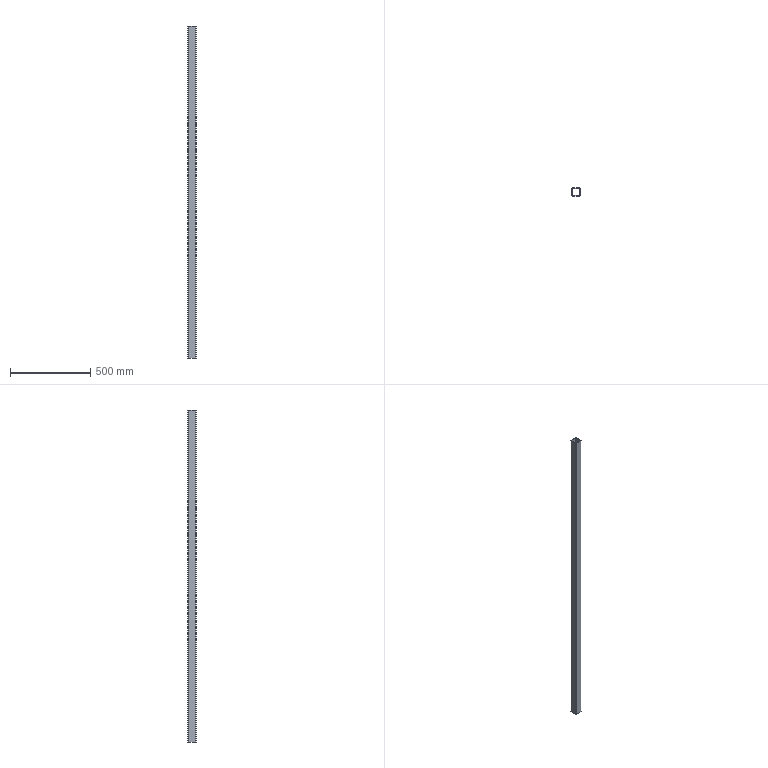Part | SolidWorks | 1 solid | 18 faces | box 50 x 50 x 2070 mm | volume 1119504 mm3 | plane 10 | cylinder 8 | commonest cylinder face diameters 6 x4 12 x4
STEP:
#1=CARTESIAN_POINT('',(19.,25.,1035.));
#2=VERTEX_POINT('',#1);
#3=CARTESIAN_POINT('',(25.,19.,1035.));
#4=VERTEX_POINT('',#3);
#5=CARTESIAN_POINT('',(19.,19.,1035.));
#6=DIRECTION('',(0.,0.,-1.));
#7=DIRECTION('',(-1.,0.,0.));
#8=AXIS2_PLACEMENT_3D('',#5,#6,#7);
#9=CIRCLE('',#8,6.);
#10=EDGE_CURVE('',#2,#4,#9,.T.);
#11=ORIENTED_EDGE('',*,*,#10,.T.);
#12=CARTESIAN_POINT('',(25.,19.,-1035.));
#13=VERTEX_POINT('',#12);
#14=CARTESIAN_POINT('',(25.,19.,-1035.));
#15=DIRECTION('',(0.,0.,1.));
#16=VECTOR('',#15,1000.);
#17=LINE('',#14,#16);
#18=EDGE_CURVE('',#13,#4,#17,.T.);
#19=ORIENTED_EDGE('',*,*,#18,.F.);
#20=CARTESIAN_POINT('',(19.,25.,-1035.));
#21=VERTEX_POINT('',#20);
#22=CARTESIAN_POINT('',(19.,19.,-1035.));
#23=DIRECTION('',(0.,0.,-1.));
#24=DIRECTION('',(-1.,0.,0.));
#25=AXIS2_PLACEMENT_3D('',#22,#23,#24);
#26=CIRCLE('',#25,6.);
#27=EDGE_CURVE('',#21,#13,#26,.T.);
#28=ORIENTED_EDGE('',*,*,#27,.F.);
#29=CARTESIAN_POINT('',(19.,25.,-1035.));
#30=DIRECTION('',(0.,0.,1.));
#31=VECTOR('',#30,1000.);
#32=LINE('',#29,#31);
#33=EDGE_CURVE('',#21,#2,#32,.T.);
#34=ORIENTED_EDGE('',*,*,#33,.T.);
#35=EDGE_LOOP('',(#11,#19,#28,#34));
#36=FACE_OUTER_BOUND('',#35,.T.);
#37=CARTESIAN_POINT('',(19.,19.,-1035.));
#38=DIRECTION('',(0.,0.,1.));
#39=DIRECTION('',(1.,0.,0.));
#40=AXIS2_PLACEMENT_3D('',#37,#38,#39);
#41=CYLINDRICAL_SURFACE('',#40,6.);
#42=ADVANCED_FACE('',(#36),#41,.T.);
#43=CARTESIAN_POINT('',(25.,-19.,1035.));
#44=VERTEX_POINT('',#43);
#45=CARTESIAN_POINT('',(25.,19.,1035.));
#46=DIRECTION('',(0.,-1.,0.));
#47=VECTOR('',#46,1000.);
#48=LINE('',#45,#47);
#49=EDGE_CURVE('',#4,#44,#48,.T.);
#50=ORIENTED_EDGE('',*,*,#49,.T.);
#51=CARTESIAN_POINT('',(25.,-19.,-1035.));
#52=VERTEX_POINT('',#51);
#53=CARTESIAN_POINT('',(25.,-19.,-1035.));
#54=DIRECTION('',(0.,0.,1.));
#55=VECTOR('',#54,1000.);
#56=LINE('',#53,#55);
#57=EDGE_CURVE('',#52,#44,#56,.T.);
#58=ORIENTED_EDGE('',*,*,#57,.F.);
#59=CARTESIAN_POINT('',(25.,19.,-1035.));
#60=DIRECTION('',(0.,-1.,0.));
#61=VECTOR('',#60,1000.);
#62=LINE('',#59,#61);
#63=EDGE_CURVE('',#13,#52,#62,.T.);
#64=ORIENTED_EDGE('',*,*,#63,.F.);
#65=ORIENTED_EDGE('',*,*,#18,.T.);
#66=EDGE_LOOP('',(#50,#58,#64,#65));
#67=FACE_OUTER_BOUND('',#66,.T.);
#68=CARTESIAN_POINT('',(25.,19.,-1035.));
#69=DIRECTION('',(-1.,0.,0.));
#70=DIRECTION('',(0.,0.,1.));
#71=AXIS2_PLACEMENT_3D('',#68,#69,#70);
#72=PLANE('',#71);
#73=ADVANCED_FACE('',(#67),#72,.F.);
#74=CARTESIAN_POINT('',(19.,-25.,1035.));
#75=VERTEX_POINT('',#74);
#76=CARTESIAN_POINT('',(19.,-19.,1035.));
#77=DIRECTION('',(0.,0.,-1.));
#78=DIRECTION('',(-1.,0.,0.));
#79=AXIS2_PLACEMENT_3D('',#76,#77,#78);
#80=CIRCLE('',#79,6.);
#81=EDGE_CURVE('',#44,#75,#80,.T.);
#82=ORIENTED_EDGE('',*,*,#81,.T.);
#83=CARTESIAN_POINT('',(19.,-25.,-1035.));
#84=VERTEX_POINT('',#83);
#85=CARTESIAN_POINT('',(19.,-25.,-1035.));
#86=DIRECTION('',(0.,0.,1.));
#87=VECTOR('',#86,1000.);
#88=LINE('',#85,#87);
#89=EDGE_CURVE('',#84,#75,#88,.T.);
#90=ORIENTED_EDGE('',*,*,#89,.F.);
#91=CARTESIAN_POINT('',(19.,-19.,-1035.));
#92=DIRECTION('',(0.,0.,-1.));
#93=DIRECTION('',(-1.,0.,0.));
#94=AXIS2_PLACEMENT_3D('',#91,#92,#93);
#95=CIRCLE('',#94,6.);
#96=EDGE_CURVE('',#52,#84,#95,.T.);
#97=ORIENTED_EDGE('',*,*,#96,.F.);
#98=ORIENTED_EDGE('',*,*,#57,.T.);
#99=EDGE_LOOP('',(#82,#90,#97,#98));
#100=FACE_OUTER_BOUND('',#99,.T.);
#101=CARTESIAN_POINT('',(19.,-19.,-1035.));
#102=DIRECTION('',(0.,0.,1.));
#103=DIRECTION('',(1.,0.,0.));
#104=AXIS2_PLACEMENT_3D('',#101,#102,#103);
#105=CYLINDRICAL_SURFACE('',#104,6.);
#106=ADVANCED_FACE('',(#100),#105,.T.);
#107=CARTESIAN_POINT('',(-19.,-25.,1035.));
#108=VERTEX_POINT('',#107);
#109=CARTESIAN_POINT('',(-19.,-25.,1035.));
#110=DIRECTION('',(-1.,0.,0.));
#111=VECTOR('',#110,1000.);
#112=LINE('',#109,#111);
#113=EDGE_CURVE('',#75,#108,#112,.T.);
#114=ORIENTED_EDGE('',*,*,#113,.T.);
#115=CARTESIAN_POINT('',(-19.,-25.,-1035.));
#116=VERTEX_POINT('',#115);
#117=CARTESIAN_POINT('',(-19.,-25.,-1035.));
#118=DIRECTION('',(0.,0.,1.));
#119=VECTOR('',#118,1000.);
#120=LINE('',#117,#119);
#121=EDGE_CURVE('',#116,#108,#120,.T.);
#122=ORIENTED_EDGE('',*,*,#121,.F.);
#123=CARTESIAN_POINT('',(-19.,-25.,-1035.));
#124=DIRECTION('',(-1.,0.,0.));
#125=VECTOR('',#124,1000.);
#126=LINE('',#123,#125);
#127=EDGE_CURVE('',#84,#116,#126,.T.);
#128=ORIENTED_EDGE('',*,*,#127,.F.);
#129=ORIENTED_EDGE('',*,*,#89,.T.);
#130=EDGE_LOOP('',(#114,#122,#128,#129));
#131=FACE_OUTER_BOUND('',#130,.T.);
#132=CARTESIAN_POINT('',(-19.,-25.,-1035.));
#133=DIRECTION('',(0.,1.,0.));
#134=DIRECTION('',(0.,0.,1.));
#135=AXIS2_PLACEMENT_3D('',#132,#133,#134);
#136=PLANE('',#135);
#137=ADVANCED_FACE('',(#131),#136,.F.);
#138=CARTESIAN_POINT('',(-25.,-19.,1035.));
#139=VERTEX_POINT('',#138);
#140=CARTESIAN_POINT('',(-19.,-19.,1035.));
#141=DIRECTION('',(0.,0.,-1.));
#142=DIRECTION('',(-1.,0.,0.));
#143=AXIS2_PLACEMENT_3D('',#140,#141,#142);
#144=CIRCLE('',#143,6.);
#145=EDGE_CURVE('',#108,#139,#144,.T.);
#146=ORIENTED_EDGE('',*,*,#145,.T.);
#147=CARTESIAN_POINT('',(-25.,-19.,-1035.));
#148=VERTEX_POINT('',#147);
#149=CARTESIAN_POINT('',(-25.,-19.,-1035.));
#150=DIRECTION('',(0.,0.,1.));
#151=VECTOR('',#150,1000.);
#152=LINE('',#149,#151);
#153=EDGE_CURVE('',#148,#139,#152,.T.);
#154=ORIENTED_EDGE('',*,*,#153,.F.);
#155=CARTESIAN_POINT('',(-19.,-19.,-1035.));
#156=DIRECTION('',(0.,0.,-1.));
#157=DIRECTION('',(-1.,0.,0.));
#158=AXIS2_PLACEMENT_3D('',#155,#156,#157);
#159=CIRCLE('',#158,6.);
#160=EDGE_CURVE('',#116,#148,#159,.T.);
#161=ORIENTED_EDGE('',*,*,#160,.F.);
#162=ORIENTED_EDGE('',*,*,#121,.T.);
#163=EDGE_LOOP('',(#146,#154,#161,#162));
#164=FACE_OUTER_BOUND('',#163,.T.);
#165=CARTESIAN_POINT('',(-19.,-19.,-1035.));
#166=DIRECTION('',(0.,0.,1.));
#167=DIRECTION('',(1.,0.,0.));
#168=AXIS2_PLACEMENT_3D('',#165,#166,#167);
#169=CYLINDRICAL_SURFACE('',#168,6.);
#170=ADVANCED_FACE('',(#164),#169,.T.);
#171=CARTESIAN_POINT('',(-25.,19.,1035.));
#172=VERTEX_POINT('',#171);
#173=CARTESIAN_POINT('',(-25.,-19.,1035.));
#174=DIRECTION('',(0.,1.,0.));
#175=VECTOR('',#174,1000.);
#176=LINE('',#173,#175);
#177=EDGE_CURVE('',#139,#172,#176,.T.);
#178=ORIENTED_EDGE('',*,*,#177,.T.);
#179=CARTESIAN_POINT('',(-25.,19.,-1035.));
#180=VERTEX_POINT('',#179);
#181=CARTESIAN_POINT('',(-25.,19.,-1035.));
#182=DIRECTION('',(0.,0.,1.));
#183=VECTOR('',#182,1000.);
#184=LINE('',#181,#183);
#185=EDGE_CURVE('',#180,#172,#184,.T.);
#186=ORIENTED_EDGE('',*,*,#185,.F.);
#187=CARTESIAN_POINT('',(-25.,-19.,-1035.));
#188=DIRECTION('',(0.,1.,0.));
#189=VECTOR('',#188,1000.);
#190=LINE('',#187,#189);
#191=EDGE_CURVE('',#148,#180,#190,.T.);
#192=ORIENTED_EDGE('',*,*,#191,.F.);
#193=ORIENTED_EDGE('',*,*,#153,.T.);
#194=EDGE_LOOP('',(#178,#186,#192,#193));
#195=FACE_OUTER_BOUND('',#194,.T.);
#196=CARTESIAN_POINT('',(-25.,-19.,-1035.));
#197=DIRECTION('',(1.,0.,0.));
#198=DIRECTION('',(0.,0.,-1.));
#199=AXIS2_PLACEMENT_3D('',#196,#197,#198);
#200=PLANE('',#199);
#201=ADVANCED_FACE('',(#195),#200,.F.);
#202=CARTESIAN_POINT('',(-19.,25.,1035.));
#203=VERTEX_POINT('',#202);
#204=CARTESIAN_POINT('',(-19.,19.,1035.));
#205=DIRECTION('',(0.,0.,-1.));
#206=DIRECTION('',(-1.,0.,0.));
#207=AXIS2_PLACEMENT_3D('',#204,#205,#206);
#208=CIRCLE('',#207,6.);
#209=EDGE_CURVE('',#172,#203,#208,.T.);
#210=ORIENTED_EDGE('',*,*,#209,.T.);
#211=CARTESIAN_POINT('',(-19.,25.,-1035.));
#212=VERTEX_POINT('',#211);
#213=CARTESIAN_POINT('',(-19.,25.,-1035.));
#214=DIRECTION('',(0.,0.,1.));
#215=VECTOR('',#214,1000.);
#216=LINE('',#213,#215);
#217=EDGE_CURVE('',#212,#203,#216,.T.);
#218=ORIENTED_EDGE('',*,*,#217,.F.);
#219=CARTESIAN_POINT('',(-19.,19.,-1035.));
#220=DIRECTION('',(0.,0.,-1.));
#221=DIRECTION('',(-1.,0.,0.));
#222=AXIS2_PLACEMENT_3D('',#219,#220,#221);
#223=CIRCLE('',#222,6.);
#224=EDGE_CURVE('',#180,#212,#223,.T.);
#225=ORIENTED_EDGE('',*,*,#224,.F.);
#226=ORIENTED_EDGE('',*,*,#185,.T.);
#227=EDGE_LOOP('',(#210,#218,#225,#226));
#228=FACE_OUTER_BOUND('',#227,.T.);
#229=CARTESIAN_POINT('',(-19.,19.,-1035.));
#230=DIRECTION('',(0.,0.,1.));
#231=DIRECTION('',(1.,0.,0.));
#232=AXIS2_PLACEMENT_3D('',#229,#230,#231);
#233=CYLINDRICAL_SURFACE('',#232,6.);
#234=ADVANCED_FACE('',(#228),#233,.T.);
#235=CARTESIAN_POINT('',(22.,-19.,1035.));
#236=VERTEX_POINT('',#235);
#237=CARTESIAN_POINT('',(19.,-22.,1035.));
#238=VERTEX_POINT('',#237);
#239=CARTESIAN_POINT('',(19.,-19.,1035.));
#240=DIRECTION('',(0.,0.,-1.));
#241=DIRECTION('',(-1.,0.,0.));
#242=AXIS2_PLACEMENT_3D('',#239,#240,#241);
#243=CIRCLE('',#242,3.);
#244=EDGE_CURVE('',#236,#238,#243,.T.);
#245=ORIENTED_EDGE('',*,*,#244,.F.);
#246=CARTESIAN_POINT('',(22.,-19.,-1035.));
#247=VERTEX_POINT('',#246);
#248=CARTESIAN_POINT('',(22.,-19.,-1035.));
#249=DIRECTION('',(0.,0.,1.));
#250=VECTOR('',#249,1000.);
#251=LINE('',#248,#250);
#252=EDGE_CURVE('',#247,#236,#251,.T.);
#253=ORIENTED_EDGE('',*,*,#252,.F.);
#254=CARTESIAN_POINT('',(19.,-22.,-1035.));
#255=VERTEX_POINT('',#254);
#256=CARTESIAN_POINT('',(19.,-19.,-1035.));
#257=DIRECTION('',(0.,0.,-1.));
#258=DIRECTION('',(-1.,0.,0.));
#259=AXIS2_PLACEMENT_3D('',#256,#257,#258);
#260=CIRCLE('',#259,3.);
#261=EDGE_CURVE('',#247,#255,#260,.T.);
#262=ORIENTED_EDGE('',*,*,#261,.T.);
#263=CARTESIAN_POINT('',(19.,-22.,-1035.));
#264=DIRECTION('',(0.,0.,1.));
#265=VECTOR('',#264,1000.);
#266=LINE('',#263,#265);
#267=EDGE_CURVE('',#255,#238,#266,.T.);
#268=ORIENTED_EDGE('',*,*,#267,.T.);
#269=EDGE_LOOP('',(#245,#253,#262,#268));
#270=FACE_OUTER_BOUND('',#269,.T.);
#271=CARTESIAN_POINT('',(19.,-19.,-1035.));
#272=DIRECTION('',(0.,0.,1.));
#273=DIRECTION('',(1.,0.,0.));
#274=AXIS2_PLACEMENT_3D('',#271,#272,#273);
#275=CYLINDRICAL_SURFACE('',#274,3.);
#276=ADVANCED_FACE('',(#270),#275,.F.);
#277=CARTESIAN_POINT('',(22.,19.,1035.));
#278=VERTEX_POINT('',#277);
#279=CARTESIAN_POINT('',(22.,19.,1035.));
#280=DIRECTION('',(0.,-1.,0.));
#281=VECTOR('',#280,1000.);
#282=LINE('',#279,#281);
#283=EDGE_CURVE('',#278,#236,#282,.T.);
#284=ORIENTED_EDGE('',*,*,#283,.F.);
#285=CARTESIAN_POINT('',(22.,19.,-1035.));
#286=VERTEX_POINT('',#285);
#287=CARTESIAN_POINT('',(22.,19.,-1035.));
#288=DIRECTION('',(0.,0.,1.));
#289=VECTOR('',#288,1000.);
#290=LINE('',#287,#289);
#291=EDGE_CURVE('',#286,#278,#290,.T.);
#292=ORIENTED_EDGE('',*,*,#291,.F.);
#293=CARTESIAN_POINT('',(22.,19.,-1035.));
#294=DIRECTION('',(0.,-1.,0.));
#295=VECTOR('',#294,1000.);
#296=LINE('',#293,#295);
#297=EDGE_CURVE('',#286,#247,#296,.T.);
#298=ORIENTED_EDGE('',*,*,#297,.T.);
#299=ORIENTED_EDGE('',*,*,#252,.T.);
#300=EDGE_LOOP('',(#284,#292,#298,#299));
#301=FACE_OUTER_BOUND('',#300,.T.);
#302=CARTESIAN_POINT('',(22.,19.,-1035.));
#303=DIRECTION('',(-1.,0.,0.));
#304=DIRECTION('',(0.,0.,1.));
#305=AXIS2_PLACEMENT_3D('',#302,#303,#304);
#306=PLANE('',#305);
#307=ADVANCED_FACE('',(#301),#306,.T.);
#308=CARTESIAN_POINT('',(19.,22.,1035.));
#309=VERTEX_POINT('',#308);
#310=CARTESIAN_POINT('',(19.,19.,1035.));
#311=DIRECTION('',(0.,0.,-1.));
#312=DIRECTION('',(-1.,0.,0.));
#313=AXIS2_PLACEMENT_3D('',#310,#311,#312);
#314=CIRCLE('',#313,3.);
#315=EDGE_CURVE('',#309,#278,#314,.T.);
#316=ORIENTED_EDGE('',*,*,#315,.F.);
#317=CARTESIAN_POINT('',(19.,22.,-1035.));
#318=VERTEX_POINT('',#317);
#319=CARTESIAN_POINT('',(19.,22.,-1035.));
#320=DIRECTION('',(0.,0.,1.));
#321=VECTOR('',#320,1000.);
#322=LINE('',#319,#321);
#323=EDGE_CURVE('',#318,#309,#322,.T.);
#324=ORIENTED_EDGE('',*,*,#323,.F.);
#325=CARTESIAN_POINT('',(19.,19.,-1035.));
#326=DIRECTION('',(0.,0.,-1.));
#327=DIRECTION('',(-1.,0.,0.));
#328=AXIS2_PLACEMENT_3D('',#325,#326,#327);
#329=CIRCLE('',#328,3.);
#330=EDGE_CURVE('',#318,#286,#329,.T.);
#331=ORIENTED_EDGE('',*,*,#330,.T.);
#332=ORIENTED_EDGE('',*,*,#291,.T.);
#333=EDGE_LOOP('',(#316,#324,#331,#332));
#334=FACE_OUTER_BOUND('',#333,.T.);
#335=CARTESIAN_POINT('',(19.,19.,-1035.));
#336=DIRECTION('',(0.,0.,1.));
#337=DIRECTION('',(1.,0.,0.));
#338=AXIS2_PLACEMENT_3D('',#335,#336,#337);
#339=CYLINDRICAL_SURFACE('',#338,3.);
#340=ADVANCED_FACE('',(#334),#339,.F.);
#341=CARTESIAN_POINT('',(-19.,22.,1035.));
#342=VERTEX_POINT('',#341);
#343=CARTESIAN_POINT('',(19.,22.,1035.));
#344=DIRECTION('',(1.,0.,0.));
#345=VECTOR('',#344,1000.);
#346=LINE('',#343,#345);
#347=EDGE_CURVE('',#342,#309,#346,.T.);
#348=ORIENTED_EDGE('',*,*,#347,.F.);
#349=CARTESIAN_POINT('',(-19.,22.,-1035.));
#350=VERTEX_POINT('',#349);
#351=CARTESIAN_POINT('',(-19.,22.,-1035.));
#352=DIRECTION('',(0.,0.,1.));
#353=VECTOR('',#352,1000.);
#354=LINE('',#351,#353);
#355=EDGE_CURVE('',#350,#342,#354,.T.);
#356=ORIENTED_EDGE('',*,*,#355,.F.);
#357=CARTESIAN_POINT('',(19.,22.,-1035.));
#358=DIRECTION('',(1.,0.,0.));
#359=VECTOR('',#358,1000.);
#360=LINE('',#357,#359);
#361=EDGE_CURVE('',#350,#318,#360,.T.);
#362=ORIENTED_EDGE('',*,*,#361,.T.);
#363=ORIENTED_EDGE('',*,*,#323,.T.);
#364=EDGE_LOOP('',(#348,#356,#362,#363));
#365=FACE_OUTER_BOUND('',#364,.T.);
#366=CARTESIAN_POINT('',(19.,22.,-1035.));
#367=DIRECTION('',(0.,-1.,0.));
#368=DIRECTION('',(0.,0.,-1.));
#369=AXIS2_PLACEMENT_3D('',#366,#367,#368);
#370=PLANE('',#369);
#371=ADVANCED_FACE('',(#365),#370,.T.);
#372=CARTESIAN_POINT('',(-22.,19.,1035.));
#373=VERTEX_POINT('',#372);
#374=CARTESIAN_POINT('',(-19.,19.,1035.));
#375=DIRECTION('',(0.,0.,-1.));
#376=DIRECTION('',(-1.,0.,0.));
#377=AXIS2_PLACEMENT_3D('',#374,#375,#376);
#378=CIRCLE('',#377,3.);
#379=EDGE_CURVE('',#373,#342,#378,.T.);
#380=ORIENTED_EDGE('',*,*,#379,.F.);
#381=CARTESIAN_POINT('',(-22.,19.,-1035.));
#382=VERTEX_POINT('',#381);
#383=CARTESIAN_POINT('',(-22.,19.,-1035.));
#384=DIRECTION('',(0.,0.,1.));
#385=VECTOR('',#384,1000.);
#386=LINE('',#383,#385);
#387=EDGE_CURVE('',#382,#373,#386,.T.);
#388=ORIENTED_EDGE('',*,*,#387,.F.);
#389=CARTESIAN_POINT('',(-19.,19.,-1035.));
#390=DIRECTION('',(0.,0.,-1.));
#391=DIRECTION('',(-1.,0.,0.));
#392=AXIS2_PLACEMENT_3D('',#389,#390,#391);
#393=CIRCLE('',#392,3.);
#394=EDGE_CURVE('',#382,#350,#393,.T.);
#395=ORIENTED_EDGE('',*,*,#394,.T.);
#396=ORIENTED_EDGE('',*,*,#355,.T.);
#397=EDGE_LOOP('',(#380,#388,#395,#396));
#398=FACE_OUTER_BOUND('',#397,.T.);
#399=CARTESIAN_POINT('',(-19.,19.,-1035.));
#400=DIRECTION('',(0.,0.,1.));
#401=DIRECTION('',(1.,0.,0.));
#402=AXIS2_PLACEMENT_3D('',#399,#400,#401);
#403=CYLINDRICAL_SURFACE('',#402,3.);
#404=ADVANCED_FACE('',(#398),#403,.F.);
#405=CARTESIAN_POINT('',(-22.,-19.,1035.));
#406=VERTEX_POINT('',#405);
#407=CARTESIAN_POINT('',(-22.,-19.,1035.));
#408=DIRECTION('',(0.,1.,0.));
#409=VECTOR('',#408,1000.);
#410=LINE('',#407,#409);
#411=EDGE_CURVE('',#406,#373,#410,.T.);
#412=ORIENTED_EDGE('',*,*,#411,.F.);
#413=CARTESIAN_POINT('',(-22.,-19.,-1035.));
#414=VERTEX_POINT('',#413);
#415=CARTESIAN_POINT('',(-22.,-19.,-1035.));
#416=DIRECTION('',(0.,0.,1.));
#417=VECTOR('',#416,1000.);
#418=LINE('',#415,#417);
#419=EDGE_CURVE('',#414,#406,#418,.T.);
#420=ORIENTED_EDGE('',*,*,#419,.F.);
#421=CARTESIAN_POINT('',(-22.,-19.,-1035.));
#422=DIRECTION('',(0.,1.,0.));
#423=VECTOR('',#422,1000.);
#424=LINE('',#421,#423);
#425=EDGE_CURVE('',#414,#382,#424,.T.);
#426=ORIENTED_EDGE('',*,*,#425,.T.);
#427=ORIENTED_EDGE('',*,*,#387,.T.);
#428=EDGE_LOOP('',(#412,#420,#426,#427));
#429=FACE_OUTER_BOUND('',#428,.T.);
#430=CARTESIAN_POINT('',(-22.,-19.,-1035.));
#431=DIRECTION('',(1.,0.,0.));
#432=DIRECTION('',(0.,0.,-1.));
#433=AXIS2_PLACEMENT_3D('',#430,#431,#432);
#434=PLANE('',#433);
#435=ADVANCED_FACE('',(#429),#434,.T.);
#436=CARTESIAN_POINT('',(-19.,-22.,1035.));
#437=VERTEX_POINT('',#436);
#438=CARTESIAN_POINT('',(-19.,-19.,1035.));
#439=DIRECTION('',(0.,0.,-1.));
#440=DIRECTION('',(-1.,0.,0.));
#441=AXIS2_PLACEMENT_3D('',#438,#439,#440);
#442=CIRCLE('',#441,3.);
#443=EDGE_CURVE('',#437,#406,#442,.T.);
#444=ORIENTED_EDGE('',*,*,#443,.F.);
#445=CARTESIAN_POINT('',(-19.,-22.,-1035.));
#446=VERTEX_POINT('',#445);
#447=CARTESIAN_POINT('',(-19.,-22.,-1035.));
#448=DIRECTION('',(0.,0.,1.));
#449=VECTOR('',#448,1000.);
#450=LINE('',#447,#449);
#451=EDGE_CURVE('',#446,#437,#450,.T.);
#452=ORIENTED_EDGE('',*,*,#451,.F.);
#453=CARTESIAN_POINT('',(-19.,-19.,-1035.));
#454=DIRECTION('',(0.,0.,-1.));
#455=DIRECTION('',(-1.,0.,0.));
#456=AXIS2_PLACEMENT_3D('',#453,#454,#455);
#457=CIRCLE('',#456,3.);
#458=EDGE_CURVE('',#446,#414,#457,.T.);
#459=ORIENTED_EDGE('',*,*,#458,.T.);
#460=ORIENTED_EDGE('',*,*,#419,.T.);
#461=EDGE_LOOP('',(#444,#452,#459,#460));
#462=FACE_OUTER_BOUND('',#461,.T.);
#463=CARTESIAN_POINT('',(-19.,-19.,-1035.));
#464=DIRECTION('',(0.,0.,1.));
#465=DIRECTION('',(1.,0.,0.));
#466=AXIS2_PLACEMENT_3D('',#463,#464,#465);
#467=CYLINDRICAL_SURFACE('',#466,3.);
#468=ADVANCED_FACE('',(#462),#467,.F.);
#469=CARTESIAN_POINT('',(-19.,-22.,1035.));
#470=DIRECTION('',(-1.,0.,0.));
#471=VECTOR('',#470,1000.);
#472=LINE('',#469,#471);
#473=EDGE_CURVE('',#238,#437,#472,.T.);
#474=ORIENTED_EDGE('',*,*,#473,.F.);
#475=ORIENTED_EDGE('',*,*,#267,.F.);
#476=CARTESIAN_POINT('',(-19.,-22.,-1035.));
#477=DIRECTION('',(-1.,0.,0.));
#478=VECTOR('',#477,1000.);
#479=LINE('',#476,#478);
#480=EDGE_CURVE('',#255,#446,#479,.T.);
#481=ORIENTED_EDGE('',*,*,#480,.T.);
#482=ORIENTED_EDGE('',*,*,#451,.T.);
#483=EDGE_LOOP('',(#474,#475,#481,#482));
#484=FACE_OUTER_BOUND('',#483,.T.);
#485=CARTESIAN_POINT('',(-19.,-22.,-1035.));
#486=DIRECTION('',(0.,1.,0.));
#487=DIRECTION('',(0.,0.,1.));
#488=AXIS2_PLACEMENT_3D('',#485,#486,#487);
#489=PLANE('',#488);
#490=ADVANCED_FACE('',(#484),#489,.T.);
#491=CARTESIAN_POINT('',(19.,25.,1035.));
#492=DIRECTION('',(1.,0.,0.));
#493=VECTOR('',#492,1000.);
#494=LINE('',#491,#493);
#495=EDGE_CURVE('',#203,#2,#494,.T.);
#496=ORIENTED_EDGE('',*,*,#495,.T.);
#497=ORIENTED_EDGE('',*,*,#33,.F.);
#498=CARTESIAN_POINT('',(19.,25.,-1035.));
#499=DIRECTION('',(1.,0.,0.));
#500=VECTOR('',#499,1000.);
#501=LINE('',#498,#500);
#502=EDGE_CURVE('',#212,#21,#501,.T.);
#503=ORIENTED_EDGE('',*,*,#502,.F.);
#504=ORIENTED_EDGE('',*,*,#217,.T.);
#505=EDGE_LOOP('',(#496,#497,#503,#504));
#506=FACE_OUTER_BOUND('',#505,.T.);
#507=CARTESIAN_POINT('',(19.,25.,-1035.));
#508=DIRECTION('',(0.,-1.,0.));
#509=DIRECTION('',(0.,0.,-1.));
#510=AXIS2_PLACEMENT_3D('',#507,#508,#509);
#511=PLANE('',#510);
#512=ADVANCED_FACE('',(#506),#511,.F.);
#513=ORIENTED_EDGE('',*,*,#261,.F.);
#514=ORIENTED_EDGE('',*,*,#297,.F.);
#515=ORIENTED_EDGE('',*,*,#330,.F.);
#516=ORIENTED_EDGE('',*,*,#361,.F.);
#517=ORIENTED_EDGE('',*,*,#394,.F.);
#518=ORIENTED_EDGE('',*,*,#425,.F.);
#519=ORIENTED_EDGE('',*,*,#458,.F.);
#520=ORIENTED_EDGE('',*,*,#480,.F.);
#521=EDGE_LOOP('',(#513,#514,#515,#516,#517,#518,#519,#520));
#522=FACE_BOUND('',#521,.T.);
#523=ORIENTED_EDGE('',*,*,#27,.T.);
#524=ORIENTED_EDGE('',*,*,#63,.T.);
#525=ORIENTED_EDGE('',*,*,#96,.T.);
#526=ORIENTED_EDGE('',*,*,#127,.T.);
#527=ORIENTED_EDGE('',*,*,#160,.T.);
#528=ORIENTED_EDGE('',*,*,#191,.T.);
#529=ORIENTED_EDGE('',*,*,#224,.T.);
#530=ORIENTED_EDGE('',*,*,#502,.T.);
#531=EDGE_LOOP('',(#523,#524,#525,#526,#527,#528,#529,#530));
#532=FACE_OUTER_BOUND('',#531,.T.);
#533=CARTESIAN_POINT('',(19.,19.,-1035.));
#534=DIRECTION('',(0.,0.,-1.));
#535=DIRECTION('',(-1.,0.,0.));
#536=AXIS2_PLACEMENT_3D('',#533,#534,#535);
#537=PLANE('',#536);
#538=ADVANCED_FACE('',(#522,#532),#537,.T.);
#539=ORIENTED_EDGE('',*,*,#244,.T.);
#540=ORIENTED_EDGE('',*,*,#473,.T.);
#541=ORIENTED_EDGE('',*,*,#443,.T.);
#542=ORIENTED_EDGE('',*,*,#411,.T.);
#543=ORIENTED_EDGE('',*,*,#379,.T.);
#544=ORIENTED_EDGE('',*,*,#347,.T.);
#545=ORIENTED_EDGE('',*,*,#315,.T.);
#546=ORIENTED_EDGE('',*,*,#283,.T.);
#547=EDGE_LOOP('',(#539,#540,#541,#542,#543,#544,#545,#546));
#548=FACE_BOUND('',#547,.T.);
#549=ORIENTED_EDGE('',*,*,#10,.F.);
#550=ORIENTED_EDGE('',*,*,#495,.F.);
#551=ORIENTED_EDGE('',*,*,#209,.F.);
#552=ORIENTED_EDGE('',*,*,#177,.F.);
#553=ORIENTED_EDGE('',*,*,#145,.F.);
#554=ORIENTED_EDGE('',*,*,#113,.F.);
#555=ORIENTED_EDGE('',*,*,#81,.F.);
#556=ORIENTED_EDGE('',*,*,#49,.F.);
#557=EDGE_LOOP('',(#549,#550,#551,#552,#553,#554,#555,#556));
#558=FACE_OUTER_BOUND('',#557,.T.);
#559=CARTESIAN_POINT('',(19.,19.,1035.));
#560=DIRECTION('',(0.,0.,-1.));
#561=DIRECTION('',(-1.,0.,0.));
#562=AXIS2_PLACEMENT_3D('',#559,#560,#561);
#563=PLANE('',#562);
#564=ADVANCED_FACE('',(#548,#558),#563,.F.);
#565=CLOSED_SHELL('',(#42,#73,#106,#137,#170,#201,#234,#276,#307,#340,#371,#404,#435,#468,#490,#512,#538,#564));
#566=MANIFOLD_SOLID_BREP('',#565);
#567=CARTESIAN_POINT('',(0.,0.,0.));
#568=DIRECTION('',(0.,0.,1.));
#569=DIRECTION('',(1.,0.,0.));
#570=AXIS2_PLACEMENT_3D('',#567,#568,#569);
#571=(LENGTH_UNIT()NAMED_UNIT(*)SI_UNIT(.MILLI.,.METRE.));
#572=UNCERTAINTY_MEASURE_WITH_UNIT(LENGTH_MEASURE(0.00001),#571,'','');
#573=(NAMED_UNIT(*)PLANE_ANGLE_UNIT()SI_UNIT($,.RADIAN.));
#574=(NAMED_UNIT(*)SI_UNIT($,.STERADIAN.)SOLID_ANGLE_UNIT());
#575=(GEOMETRIC_REPRESENTATION_CONTEXT(3)GLOBAL_UNCERTAINTY_ASSIGNED_CONTEXT((#572))GLOBAL_UNIT_ASSIGNED_CONTEXT((#571,#573,#574))REPRESENTATION_CONTEXT('',''));
#576=ADVANCED_BREP_SHAPE_REPRESENTATION('',(#566,#570),#575);